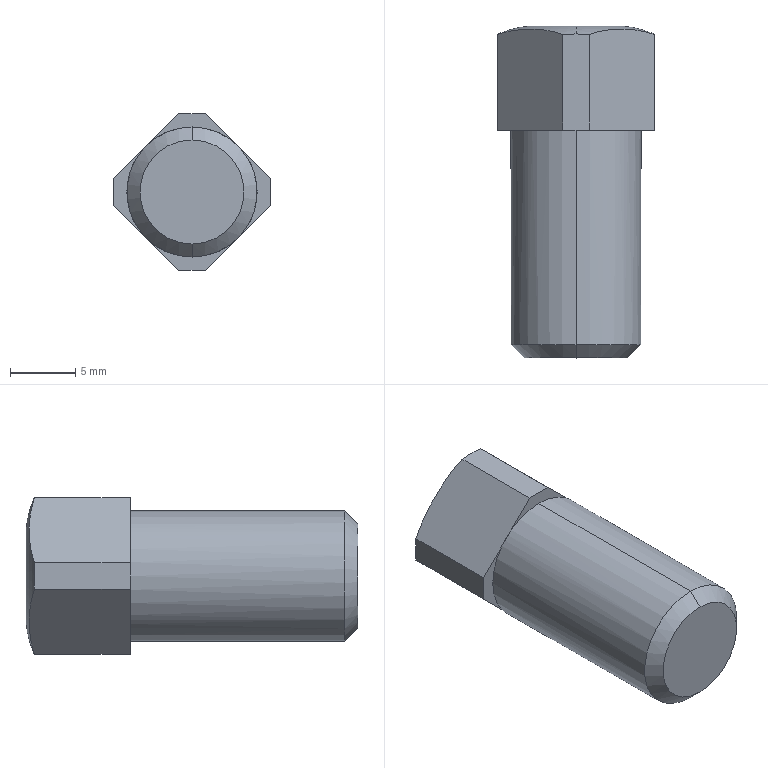Part | SolidWorks | features Chamfer 2, ICE 2, RevCut 1, Revolution 1 | 1 solid | 24 faces | box 12 x 25.5 x 12 mm | volume 2101 mm3 | plane 18 | cone 2 | torus 2 | cylinder 2 | commonest cylinder face diameters 10 x2
STEP:
#1=CARTESIAN_POINT('',(0.,-1.5,-4.));
#2=VERTEX_POINT('',#1);
#3=CARTESIAN_POINT('',(0.,-1.5,4.));
#4=VERTEX_POINT('',#3);
#5=CARTESIAN_POINT('',(0.,-1.5,0.));
#6=DIRECTION('',(0.,-1.,0.));
#7=DIRECTION('',(0.,0.,-1.));
#8=AXIS2_PLACEMENT_3D('',#5,#6,#7);
#9=CIRCLE('',#8,4.);
#10=EDGE_CURVE('',#2,#4,#9,.T.);
#11=ORIENTED_EDGE('',*,*,#10,.F.);
#12=CARTESIAN_POINT('',(0.,-0.5,-5.));
#13=VERTEX_POINT('',#12);
#14=CARTESIAN_POINT('',(0.,-1.5,-4.));
#15=DIRECTION('',(0.,0.7071,-0.7071));
#16=VECTOR('',#15,1000.);
#17=LINE('',#14,#16);
#18=EDGE_CURVE('',#2,#13,#17,.T.);
#19=ORIENTED_EDGE('',*,*,#18,.T.);
#20=CARTESIAN_POINT('',(0.,-0.5,5.));
#21=VERTEX_POINT('',#20);
#22=CARTESIAN_POINT('',(0.,-0.5,0.));
#23=DIRECTION('',(0.,1.,0.));
#24=DIRECTION('',(0.,0.,-1.));
#25=AXIS2_PLACEMENT_3D('',#22,#23,#24);
#26=CIRCLE('',#25,5.);
#27=EDGE_CURVE('',#21,#13,#26,.T.);
#28=ORIENTED_EDGE('',*,*,#27,.F.);
#29=CARTESIAN_POINT('',(0.,-1.5,4.));
#30=DIRECTION('',(0.,0.7071,0.7071));
#31=VECTOR('',#30,1000.);
#32=LINE('',#29,#31);
#33=EDGE_CURVE('',#4,#21,#32,.T.);
#34=ORIENTED_EDGE('',*,*,#33,.F.);
#35=EDGE_LOOP('',(#11,#19,#28,#34));
#36=FACE_OUTER_BOUND('',#35,.T.);
#37=CARTESIAN_POINT('',(0.,-1.5,0.));
#38=DIRECTION('',(0.,1.,0.));
#39=DIRECTION('',(0.,0.,1.));
#40=AXIS2_PLACEMENT_3D('',#37,#38,#39);
#41=CONICAL_SURFACE('',#40,4.,0.7854);
#42=ADVANCED_FACE('',(#36),#41,.T.);
#43=CARTESIAN_POINT('',(0.,24.,-3.5));
#44=VERTEX_POINT('',#43);
#45=CARTESIAN_POINT('',(0.,24.,3.5));
#46=VERTEX_POINT('',#45);
#47=CARTESIAN_POINT('',(0.,24.,0.));
#48=DIRECTION('',(0.,-1.,0.));
#49=DIRECTION('',(0.,0.,-1.));
#50=AXIS2_PLACEMENT_3D('',#47,#48,#49);
#51=CIRCLE('',#50,3.5);
#52=EDGE_CURVE('',#44,#46,#51,.T.);
#53=ORIENTED_EDGE('',*,*,#52,.T.);
#54=CARTESIAN_POINT('',(0.,23.385,6.));
#55=VERTEX_POINT('',#54);
#56=CARTESIAN_POINT('',(0.,16.602,3.006));
#57=DIRECTION('',(1.,0.,0.));
#58=DIRECTION('',(0.,0.,-1.));
#59=AXIS2_PLACEMENT_3D('',#56,#57,#58);
#60=CIRCLE('',#59,7.415);
#61=EDGE_CURVE('',#46,#55,#60,.T.);
#62=ORIENTED_EDGE('',*,*,#61,.T.);
#63=CARTESIAN_POINT('',(1.,23.348,6.));
#64=VERTEX_POINT('',#63);
#65=CARTESIAN_POINT('',(0.,23.385,6.));
#66=CARTESIAN_POINT('',(0.1677,23.385,6.));
#67=CARTESIAN_POINT('',(0.5021,23.379,6.));
#68=CARTESIAN_POINT('',(0.8344,23.36,6.));
#69=CARTESIAN_POINT('',(1.,23.348,6.));
#70=B_SPLINE_CURVE_WITH_KNOTS('',3,(#65,#66,#67,#68,#69),.UNSPECIFIED.,.F.,.F.,(4,1,4),(0.,0.0004963,0.0009926),.UNSPECIFIED.);
#71=EDGE_CURVE('',#55,#64,#70,.T.);
#72=ORIENTED_EDGE('',*,*,#71,.T.);
#73=CARTESIAN_POINT('',(6.,23.348,1.));
#74=VERTEX_POINT('',#73);
#75=CARTESIAN_POINT('',(1.,23.348,6.));
#76=CARTESIAN_POINT('',(1.411,23.502,5.589));
#77=CARTESIAN_POINT('',(1.825,23.602,5.175));
#78=CARTESIAN_POINT('',(2.657,23.729,4.343));
#79=CARTESIAN_POINT('',(3.075,23.757,3.925));
#80=CARTESIAN_POINT('',(3.915,23.757,3.085));
#81=CARTESIAN_POINT('',(4.339,23.73,2.661));
#82=CARTESIAN_POINT('',(5.176,23.602,1.824));
#83=CARTESIAN_POINT('',(5.591,23.501,1.409));
#84=CARTESIAN_POINT('',(6.,23.348,1.));
#85=B_SPLINE_CURVE_WITH_KNOTS('',3,(#75,#76,#77,#78,#79,#80,#81,#82,#83,#84),.UNSPECIFIED.,.F.,.F.,(4,2,2,2,4),(0.000000288,0.001776,0.003551,0.005327,0.007102),.UNSPECIFIED.);
#86=EDGE_CURVE('',#64,#74,#85,.T.);
#87=ORIENTED_EDGE('',*,*,#86,.T.);
#88=CARTESIAN_POINT('',(6.,23.348,-1.));
#89=VERTEX_POINT('',#88);
#90=CARTESIAN_POINT('',(6.,23.348,1.));
#91=CARTESIAN_POINT('',(6.,23.373,0.6665));
#92=CARTESIAN_POINT('',(6.,23.385,0.3303));
#93=CARTESIAN_POINT('',(6.,23.385,-0.3379));
#94=CARTESIAN_POINT('',(6.,23.373,-0.67));
#95=CARTESIAN_POINT('',(6.,23.348,-1.));
#96=B_SPLINE_CURVE_WITH_KNOTS('',3,(#90,#91,#92,#93,#94,#95),.UNSPECIFIED.,.F.,.F.,(4,2,4),(0.04716,0.04814,0.04913),.UNSPECIFIED.);
#97=EDGE_CURVE('',#74,#89,#96,.T.);
#98=ORIENTED_EDGE('',*,*,#97,.T.);
#99=CARTESIAN_POINT('',(1.,23.348,-6.));
#100=VERTEX_POINT('',#99);
#101=CARTESIAN_POINT('',(6.,23.348,-1.));
#102=CARTESIAN_POINT('',(5.589,23.502,-1.411));
#103=CARTESIAN_POINT('',(5.175,23.602,-1.825));
#104=CARTESIAN_POINT('',(4.343,23.729,-2.657));
#105=CARTESIAN_POINT('',(3.925,23.757,-3.075));
#106=CARTESIAN_POINT('',(3.085,23.757,-3.915));
#107=CARTESIAN_POINT('',(2.661,23.73,-4.339));
#108=CARTESIAN_POINT('',(1.824,23.602,-5.176));
#109=CARTESIAN_POINT('',(1.409,23.501,-5.591));
#110=CARTESIAN_POINT('',(1.,23.348,-6.));
#111=B_SPLINE_CURVE_WITH_KNOTS('',3,(#101,#102,#103,#104,#105,#106,#107,#108,#109,#110),.UNSPECIFIED.,.F.,.F.,(4,2,2,2,4),(0.000000288,0.001776,0.003551,0.005327,0.007102),.UNSPECIFIED.);
#112=EDGE_CURVE('',#89,#100,#111,.T.);
#113=ORIENTED_EDGE('',*,*,#112,.T.);
#114=CARTESIAN_POINT('',(0.,23.385,-6.));
#115=VERTEX_POINT('',#114);
#116=CARTESIAN_POINT('',(1.,23.348,-6.));
#117=CARTESIAN_POINT('',(0.8339,23.36,-6.));
#118=CARTESIAN_POINT('',(0.6675,23.37,-6.));
#119=CARTESIAN_POINT('',(0.3342,23.382,-6.));
#120=CARTESIAN_POINT('',(0.1664,23.385,-6.));
#121=CARTESIAN_POINT('',(0.,23.385,-6.));
#122=B_SPLINE_CURVE_WITH_KNOTS('',3,(#116,#117,#118,#119,#120,#121),.UNSPECIFIED.,.F.,.F.,(4,2,4),(0.04716,0.04765,0.04814),.UNSPECIFIED.);
#123=EDGE_CURVE('',#100,#115,#122,.T.);
#124=ORIENTED_EDGE('',*,*,#123,.T.);
#125=CARTESIAN_POINT('',(0.,16.602,-3.006));
#126=DIRECTION('',(-1.,0.,0.));
#127=DIRECTION('',(0.,0.,1.));
#128=AXIS2_PLACEMENT_3D('',#125,#126,#127);
#129=CIRCLE('',#128,7.415);
#130=EDGE_CURVE('',#44,#115,#129,.T.);
#131=ORIENTED_EDGE('',*,*,#130,.F.);
#132=EDGE_LOOP('',(#53,#62,#72,#87,#98,#113,#124,#131));
#133=FACE_OUTER_BOUND('',#132,.T.);
#134=CARTESIAN_POINT('',(0.,16.602,0.));
#135=DIRECTION('',(0.,-1.,0.));
#136=DIRECTION('',(0.,0.,-1.));
#137=AXIS2_PLACEMENT_3D('',#134,#135,#136);
#138=TOROIDAL_SURFACE('',#137,3.006,7.415);
#139=ADVANCED_FACE('',(#133),#138,.T.);
#140=CARTESIAN_POINT('',(3.,16.,4.));
#141=VERTEX_POINT('',#140);
#142=CARTESIAN_POINT('',(0.,16.,5.));
#143=VERTEX_POINT('',#142);
#144=CARTESIAN_POINT('',(0.,16.,0.));
#145=DIRECTION('',(0.,-1.,0.));
#146=DIRECTION('',(0.,0.,-1.));
#147=AXIS2_PLACEMENT_3D('',#144,#145,#146);
#148=CIRCLE('',#147,5.);
#149=EDGE_CURVE('',#141,#143,#148,.T.);
#150=ORIENTED_EDGE('',*,*,#149,.T.);
#151=CARTESIAN_POINT('',(0.,0.,5.));
#152=DIRECTION('',(0.,-1.,0.));
#153=VECTOR('',#152,1000.);
#154=LINE('',#151,#153);
#155=EDGE_CURVE('',#143,#21,#154,.T.);
#156=ORIENTED_EDGE('',*,*,#155,.T.);
#157=ORIENTED_EDGE('',*,*,#27,.T.);
#158=CARTESIAN_POINT('',(0.,16.,-5.));
#159=VERTEX_POINT('',#158);
#160=CARTESIAN_POINT('',(0.,0.,-5.));
#161=DIRECTION('',(0.,-1.,0.));
#162=VECTOR('',#161,1000.);
#163=LINE('',#160,#162);
#164=EDGE_CURVE('',#159,#13,#163,.T.);
#165=ORIENTED_EDGE('',*,*,#164,.F.);
#166=CARTESIAN_POINT('',(3.,16.,-4.));
#167=VERTEX_POINT('',#166);
#168=CARTESIAN_POINT('',(0.,16.,0.));
#169=DIRECTION('',(0.,-1.,0.));
#170=DIRECTION('',(0.,0.,-1.));
#171=AXIS2_PLACEMENT_3D('',#168,#169,#170);
#172=CIRCLE('',#171,5.);
#173=EDGE_CURVE('',#159,#167,#172,.T.);
#174=ORIENTED_EDGE('',*,*,#173,.T.);
#175=CARTESIAN_POINT('',(4.,16.,-3.));
#176=VERTEX_POINT('',#175);
#177=CARTESIAN_POINT('',(0.,16.,0.));
#178=DIRECTION('',(0.,-1.,0.));
#179=DIRECTION('',(0.,0.,-1.));
#180=AXIS2_PLACEMENT_3D('',#177,#178,#179);
#181=CIRCLE('',#180,5.);
#182=EDGE_CURVE('',#167,#176,#181,.T.);
#183=ORIENTED_EDGE('',*,*,#182,.T.);
#184=CARTESIAN_POINT('',(4.,16.,3.));
#185=VERTEX_POINT('',#184);
#186=CARTESIAN_POINT('',(0.,16.,0.));
#187=DIRECTION('',(0.,-1.,0.));
#188=DIRECTION('',(0.,0.,-1.));
#189=AXIS2_PLACEMENT_3D('',#186,#187,#188);
#190=CIRCLE('',#189,5.);
#191=EDGE_CURVE('',#176,#185,#190,.T.);
#192=ORIENTED_EDGE('',*,*,#191,.T.);
#193=CARTESIAN_POINT('',(0.,16.,0.));
#194=DIRECTION('',(0.,-1.,0.));
#195=DIRECTION('',(0.,0.,-1.));
#196=AXIS2_PLACEMENT_3D('',#193,#194,#195);
#197=CIRCLE('',#196,5.);
#198=EDGE_CURVE('',#185,#141,#197,.T.);
#199=ORIENTED_EDGE('',*,*,#198,.T.);
#200=EDGE_LOOP('',(#150,#156,#157,#165,#174,#183,#192,#199));
#201=FACE_OUTER_BOUND('',#200,.T.);
#202=CARTESIAN_POINT('',(0.,0.,0.));
#203=DIRECTION('',(0.,-1.,0.));
#204=DIRECTION('',(0.,0.,-1.));
#205=AXIS2_PLACEMENT_3D('',#202,#203,#204);
#206=CYLINDRICAL_SURFACE('',#205,5.);
#207=ADVANCED_FACE('',(#201),#206,.T.);
#208=CARTESIAN_POINT('',(-3.,16.,-4.));
#209=VERTEX_POINT('',#208);
#210=CARTESIAN_POINT('',(0.,16.,0.));
#211=DIRECTION('',(0.,-1.,0.));
#212=DIRECTION('',(0.,0.,-1.));
#213=AXIS2_PLACEMENT_3D('',#210,#211,#212);
#214=CIRCLE('',#213,5.);
#215=EDGE_CURVE('',#209,#159,#214,.T.);
#216=ORIENTED_EDGE('',*,*,#215,.F.);
#217=CARTESIAN_POINT('',(-1.,16.,-6.));
#218=VERTEX_POINT('',#217);
#219=CARTESIAN_POINT('',(-1.,16.,-6.));
#220=DIRECTION('',(-0.7071,0.,0.7071));
#221=VECTOR('',#220,1000.);
#222=LINE('',#219,#221);
#223=EDGE_CURVE('',#218,#209,#222,.T.);
#224=ORIENTED_EDGE('',*,*,#223,.F.);
#225=CARTESIAN_POINT('',(1.,16.,-6.));
#226=VERTEX_POINT('',#225);
#227=CARTESIAN_POINT('',(-1.,16.,-6.));
#228=DIRECTION('',(-1.,0.,0.));
#229=VECTOR('',#228,1000.);
#230=LINE('',#227,#229);
#231=EDGE_CURVE('',#226,#218,#230,.T.);
#232=ORIENTED_EDGE('',*,*,#231,.F.);
#233=CARTESIAN_POINT('',(6.,16.,-1.));
#234=DIRECTION('',(-0.7071,0.,-0.7071));
#235=VECTOR('',#234,1000.);
#236=LINE('',#233,#235);
#237=EDGE_CURVE('',#167,#226,#236,.T.);
#238=ORIENTED_EDGE('',*,*,#237,.F.);
#239=ORIENTED_EDGE('',*,*,#173,.F.);
#240=EDGE_LOOP('',(#216,#224,#232,#238,#239));
#241=FACE_OUTER_BOUND('',#240,.T.);
#242=CARTESIAN_POINT('',(10.,16.,0.));
#243=DIRECTION('',(0.,-1.,0.));
#244=DIRECTION('',(0.,0.,-1.));
#245=AXIS2_PLACEMENT_3D('',#242,#243,#244);
#246=PLANE('',#245);
#247=ADVANCED_FACE('',(#241),#246,.T.);
#248=ORIENTED_EDGE('',*,*,#191,.F.);
#249=CARTESIAN_POINT('',(6.,16.,-1.));
#250=VERTEX_POINT('',#249);
#251=CARTESIAN_POINT('',(6.,16.,-1.));
#252=DIRECTION('',(-0.7071,0.,-0.7071));
#253=VECTOR('',#252,1000.);
#254=LINE('',#251,#253);
#255=EDGE_CURVE('',#250,#176,#254,.T.);
#256=ORIENTED_EDGE('',*,*,#255,.F.);
#257=CARTESIAN_POINT('',(6.,16.,1.));
#258=VERTEX_POINT('',#257);
#259=CARTESIAN_POINT('',(6.,16.,-1.));
#260=DIRECTION('',(0.,0.,-1.));
#261=VECTOR('',#260,1000.);
#262=LINE('',#259,#261);
#263=EDGE_CURVE('',#258,#250,#262,.T.);
#264=ORIENTED_EDGE('',*,*,#263,.F.);
#265=CARTESIAN_POINT('',(6.,16.,1.));
#266=DIRECTION('',(0.7071,0.,-0.7071));
#267=VECTOR('',#266,1000.);
#268=LINE('',#265,#267);
#269=EDGE_CURVE('',#185,#258,#268,.T.);
#270=ORIENTED_EDGE('',*,*,#269,.F.);
#271=EDGE_LOOP('',(#248,#256,#264,#270));
#272=FACE_OUTER_BOUND('',#271,.T.);
#273=CARTESIAN_POINT('',(10.,16.,0.));
#274=DIRECTION('',(0.,-1.,0.));
#275=DIRECTION('',(0.,0.,-1.));
#276=AXIS2_PLACEMENT_3D('',#273,#274,#275);
#277=PLANE('',#276);
#278=ADVANCED_FACE('',(#272),#277,.T.);
#279=ORIENTED_EDGE('',*,*,#149,.F.);
#280=CARTESIAN_POINT('',(1.,16.,6.));
#281=VERTEX_POINT('',#280);
#282=CARTESIAN_POINT('',(6.,16.,1.));
#283=DIRECTION('',(0.7071,0.,-0.7071));
#284=VECTOR('',#283,1000.);
#285=LINE('',#282,#284);
#286=EDGE_CURVE('',#281,#141,#285,.T.);
#287=ORIENTED_EDGE('',*,*,#286,.F.);
#288=CARTESIAN_POINT('',(-1.,16.,6.));
#289=VERTEX_POINT('',#288);
#290=CARTESIAN_POINT('',(-1.,16.,6.));
#291=DIRECTION('',(1.,0.,0.));
#292=VECTOR('',#291,1000.);
#293=LINE('',#290,#292);
#294=EDGE_CURVE('',#289,#281,#293,.T.);
#295=ORIENTED_EDGE('',*,*,#294,.F.);
#296=CARTESIAN_POINT('',(-3.,16.,4.));
#297=VERTEX_POINT('',#296);
#298=CARTESIAN_POINT('',(-1.,16.,6.));
#299=DIRECTION('',(0.7071,0.,0.7071));
#300=VECTOR('',#299,1000.);
#301=LINE('',#298,#300);
#302=EDGE_CURVE('',#297,#289,#301,.T.);
#303=ORIENTED_EDGE('',*,*,#302,.F.);
#304=CARTESIAN_POINT('',(0.,16.,0.));
#305=DIRECTION('',(0.,-1.,0.));
#306=DIRECTION('',(0.,0.,-1.));
#307=AXIS2_PLACEMENT_3D('',#304,#305,#306);
#308=CIRCLE('',#307,5.);
#309=EDGE_CURVE('',#143,#297,#308,.T.);
#310=ORIENTED_EDGE('',*,*,#309,.F.);
#311=EDGE_LOOP('',(#279,#287,#295,#303,#310));
#312=FACE_OUTER_BOUND('',#311,.T.);
#313=CARTESIAN_POINT('',(10.,16.,0.));
#314=DIRECTION('',(0.,-1.,0.));
#315=DIRECTION('',(0.,0.,-1.));
#316=AXIS2_PLACEMENT_3D('',#313,#314,#315);
#317=PLANE('',#316);
#318=ADVANCED_FACE('',(#312),#317,.T.);
#319=CARTESIAN_POINT('',(-6.,16.,-1.));
#320=VERTEX_POINT('',#319);
#321=CARTESIAN_POINT('',(-6.,16.,1.));
#322=VERTEX_POINT('',#321);
#323=CARTESIAN_POINT('',(-6.,16.,-1.));
#324=DIRECTION('',(0.,0.,1.));
#325=VECTOR('',#324,1000.);
#326=LINE('',#323,#325);
#327=EDGE_CURVE('',#320,#322,#326,.T.);
#328=ORIENTED_EDGE('',*,*,#327,.F.);
#329=CARTESIAN_POINT('',(-4.,16.,-3.));
#330=VERTEX_POINT('',#329);
#331=CARTESIAN_POINT('',(-1.,16.,-6.));
#332=DIRECTION('',(-0.7071,0.,0.7071));
#333=VECTOR('',#332,1000.);
#334=LINE('',#331,#333);
#335=EDGE_CURVE('',#330,#320,#334,.T.);
#336=ORIENTED_EDGE('',*,*,#335,.F.);
#337=CARTESIAN_POINT('',(-4.,16.,3.));
#338=VERTEX_POINT('',#337);
#339=CARTESIAN_POINT('',(0.,16.,0.));
#340=DIRECTION('',(0.,-1.,0.));
#341=DIRECTION('',(0.,0.,-1.));
#342=AXIS2_PLACEMENT_3D('',#339,#340,#341);
#343=CIRCLE('',#342,5.);
#344=EDGE_CURVE('',#338,#330,#343,.T.);
#345=ORIENTED_EDGE('',*,*,#344,.F.);
#346=CARTESIAN_POINT('',(-1.,16.,6.));
#347=DIRECTION('',(0.7071,0.,0.7071));
#348=VECTOR('',#347,1000.);
#349=LINE('',#346,#348);
#350=EDGE_CURVE('',#322,#338,#349,.T.);
#351=ORIENTED_EDGE('',*,*,#350,.F.);
#352=EDGE_LOOP('',(#328,#336,#345,#351));
#353=FACE_OUTER_BOUND('',#352,.T.);
#354=CARTESIAN_POINT('',(10.,16.,0.));
#355=DIRECTION('',(0.,-1.,0.));
#356=DIRECTION('',(0.,0.,-1.));
#357=AXIS2_PLACEMENT_3D('',#354,#355,#356);
#358=PLANE('',#357);
#359=ADVANCED_FACE('',(#353),#358,.T.);
#360=ORIENTED_EDGE('',*,*,#155,.F.);
#361=ORIENTED_EDGE('',*,*,#309,.T.);
#362=CARTESIAN_POINT('',(0.,16.,0.));
#363=DIRECTION('',(0.,-1.,0.));
#364=DIRECTION('',(0.,0.,-1.));
#365=AXIS2_PLACEMENT_3D('',#362,#363,#364);
#366=CIRCLE('',#365,5.);
#367=EDGE_CURVE('',#297,#338,#366,.T.);
#368=ORIENTED_EDGE('',*,*,#367,.T.);
#369=ORIENTED_EDGE('',*,*,#344,.T.);
#370=CARTESIAN_POINT('',(0.,16.,0.));
#371=DIRECTION('',(0.,-1.,0.));
#372=DIRECTION('',(0.,0.,-1.));
#373=AXIS2_PLACEMENT_3D('',#370,#371,#372);
#374=CIRCLE('',#373,5.);
#375=EDGE_CURVE('',#330,#209,#374,.T.);
#376=ORIENTED_EDGE('',*,*,#375,.T.);
#377=ORIENTED_EDGE('',*,*,#215,.T.);
#378=ORIENTED_EDGE('',*,*,#164,.T.);
#379=CARTESIAN_POINT('',(0.,-0.5,0.));
#380=DIRECTION('',(0.,1.,0.));
#381=DIRECTION('',(0.,0.,-1.));
#382=AXIS2_PLACEMENT_3D('',#379,#380,#381);
#383=CIRCLE('',#382,5.);
#384=EDGE_CURVE('',#13,#21,#383,.T.);
#385=ORIENTED_EDGE('',*,*,#384,.T.);
#386=EDGE_LOOP('',(#360,#361,#368,#369,#376,#377,#378,#385));
#387=FACE_OUTER_BOUND('',#386,.T.);
#388=CARTESIAN_POINT('',(0.,0.,0.));
#389=DIRECTION('',(0.,-1.,0.));
#390=DIRECTION('',(0.,0.,-1.));
#391=AXIS2_PLACEMENT_3D('',#388,#389,#390);
#392=CYLINDRICAL_SURFACE('',#391,5.);
#393=ADVANCED_FACE('',(#387),#392,.T.);
#394=ORIENTED_EDGE('',*,*,#375,.F.);
#395=CARTESIAN_POINT('',(-1.,16.,-6.));
#396=DIRECTION('',(-0.7071,0.,0.7071));
#397=VECTOR('',#396,1000.);
#398=LINE('',#395,#397);
#399=EDGE_CURVE('',#209,#330,#398,.T.);
#400=ORIENTED_EDGE('',*,*,#399,.F.);
#401=EDGE_LOOP('',(#394,#400));
#402=FACE_OUTER_BOUND('',#401,.T.);
#403=CARTESIAN_POINT('',(10.,16.,0.));
#404=DIRECTION('',(0.,-1.,0.));
#405=DIRECTION('',(0.,0.,-1.));
#406=AXIS2_PLACEMENT_3D('',#403,#404,#405);
#407=PLANE('',#406);
#408=ADVANCED_FACE('',(#402),#407,.F.);
#409=ORIENTED_EDGE('',*,*,#367,.F.);
#410=CARTESIAN_POINT('',(-1.,16.,6.));
#411=DIRECTION('',(0.7071,0.,0.7071));
#412=VECTOR('',#411,1000.);
#413=LINE('',#410,#412);
#414=EDGE_CURVE('',#338,#297,#413,.T.);
#415=ORIENTED_EDGE('',*,*,#414,.F.);
#416=EDGE_LOOP('',(#409,#415));
#417=FACE_OUTER_BOUND('',#416,.T.);
#418=CARTESIAN_POINT('',(10.,16.,0.));
#419=DIRECTION('',(0.,-1.,0.));
#420=DIRECTION('',(0.,0.,-1.));
#421=AXIS2_PLACEMENT_3D('',#418,#419,#420);
#422=PLANE('',#421);
#423=ADVANCED_FACE('',(#417),#422,.F.);
#424=ORIENTED_EDGE('',*,*,#198,.F.);
#425=CARTESIAN_POINT('',(6.,16.,1.));
#426=DIRECTION('',(0.7071,0.,-0.7071));
#427=VECTOR('',#426,1000.);
#428=LINE('',#425,#427);
#429=EDGE_CURVE('',#141,#185,#428,.T.);
#430=ORIENTED_EDGE('',*,*,#429,.F.);
#431=EDGE_LOOP('',(#424,#430));
#432=FACE_OUTER_BOUND('',#431,.T.);
#433=CARTESIAN_POINT('',(10.,16.,0.));
#434=DIRECTION('',(0.,-1.,0.));
#435=DIRECTION('',(0.,0.,-1.));
#436=AXIS2_PLACEMENT_3D('',#433,#434,#435);
#437=PLANE('',#436);
#438=ADVANCED_FACE('',(#432),#437,.F.);
#439=CARTESIAN_POINT('',(-1.,23.348,-6.));
#440=VERTEX_POINT('',#439);
#441=CARTESIAN_POINT('',(-6.,23.348,-1.));
#442=VERTEX_POINT('',#441);
#443=CARTESIAN_POINT('',(-1.,23.348,-6.));
#444=CARTESIAN_POINT('',(-1.411,23.502,-5.589));
#445=CARTESIAN_POINT('',(-1.825,23.602,-5.175));
#446=CARTESIAN_POINT('',(-2.657,23.729,-4.343));
#447=CARTESIAN_POINT('',(-3.075,23.757,-3.925));
#448=CARTESIAN_POINT('',(-3.915,23.757,-3.085));
#449=CARTESIAN_POINT('',(-4.339,23.73,-2.661));
#450=CARTESIAN_POINT('',(-5.176,23.602,-1.824));
#451=CARTESIAN_POINT('',(-5.591,23.501,-1.409));
#452=CARTESIAN_POINT('',(-6.,23.348,-1.));
#453=B_SPLINE_CURVE_WITH_KNOTS('',3,(#443,#444,#445,#446,#447,#448,#449,#450,#451,#452),.UNSPECIFIED.,.F.,.F.,(4,2,2,2,4),(0.000000288,0.001776,0.003551,0.005327,0.007102),.UNSPECIFIED.);
#454=EDGE_CURVE('',#440,#442,#453,.T.);
#455=ORIENTED_EDGE('',*,*,#454,.F.);
#456=CARTESIAN_POINT('',(-1.,-17.879,-6.));
#457=DIRECTION('',(0.,1.,0.));
#458=VECTOR('',#457,1000.);
#459=LINE('',#456,#458);
#460=EDGE_CURVE('',#218,#440,#459,.T.);
#461=ORIENTED_EDGE('',*,*,#460,.F.);
#462=ORIENTED_EDGE('',*,*,#223,.T.);
#463=ORIENTED_EDGE('',*,*,#399,.T.);
#464=ORIENTED_EDGE('',*,*,#335,.T.);
#465=CARTESIAN_POINT('',(-6.,-17.879,-1.));
#466=DIRECTION('',(0.,1.,0.));
#467=VECTOR('',#466,1000.);
#468=LINE('',#465,#467);
#469=EDGE_CURVE('',#320,#442,#468,.T.);
#470=ORIENTED_EDGE('',*,*,#469,.T.);
#471=EDGE_LOOP('',(#455,#461,#462,#463,#464,#470));
#472=FACE_OUTER_BOUND('',#471,.T.);
#473=CARTESIAN_POINT('',(-1.,-17.879,-6.));
#474=DIRECTION('',(-0.7071,0.,-0.7071));
#475=DIRECTION('',(-0.7071,0.,0.7071));
#476=AXIS2_PLACEMENT_3D('',#473,#474,#475);
#477=PLANE('',#476);
#478=ADVANCED_FACE('',(#472),#477,.T.);
#479=ORIENTED_EDGE('',*,*,#123,.F.);
#480=CARTESIAN_POINT('',(1.,-17.879,-6.));
#481=DIRECTION('',(0.,1.,0.));
#482=VECTOR('',#481,1000.);
#483=LINE('',#480,#482);
#484=EDGE_CURVE('',#226,#100,#483,.T.);
#485=ORIENTED_EDGE('',*,*,#484,.F.);
#486=ORIENTED_EDGE('',*,*,#231,.T.);
#487=ORIENTED_EDGE('',*,*,#460,.T.);
#488=CARTESIAN_POINT('',(0.,23.385,-6.));
#489=CARTESIAN_POINT('',(-0.1677,23.385,-6.));
#490=CARTESIAN_POINT('',(-0.5021,23.379,-6.));
#491=CARTESIAN_POINT('',(-0.8344,23.36,-6.));
#492=CARTESIAN_POINT('',(-1.,23.348,-6.));
#493=B_SPLINE_CURVE_WITH_KNOTS('',3,(#488,#489,#490,#491,#492),.UNSPECIFIED.,.F.,.F.,(4,1,4),(0.,0.0004963,0.0009926),.UNSPECIFIED.);
#494=EDGE_CURVE('',#115,#440,#493,.T.);
#495=ORIENTED_EDGE('',*,*,#494,.F.);
#496=EDGE_LOOP('',(#479,#485,#486,#487,#495));
#497=FACE_OUTER_BOUND('',#496,.T.);
#498=CARTESIAN_POINT('',(-1.,-17.879,-6.));
#499=DIRECTION('',(0.,0.,-1.));
#500=DIRECTION('',(-1.,0.,0.));
#501=AXIS2_PLACEMENT_3D('',#498,#499,#500);
#502=PLANE('',#501);
#503=ADVANCED_FACE('',(#497),#502,.T.);
#504=ORIENTED_EDGE('',*,*,#112,.F.);
#505=CARTESIAN_POINT('',(6.,-17.879,-1.));
#506=DIRECTION('',(0.,1.,0.));
#507=VECTOR('',#506,1000.);
#508=LINE('',#505,#507);
#509=EDGE_CURVE('',#250,#89,#508,.T.);
#510=ORIENTED_EDGE('',*,*,#509,.F.);
#511=ORIENTED_EDGE('',*,*,#255,.T.);
#512=CARTESIAN_POINT('',(6.,16.,-1.));
#513=DIRECTION('',(-0.7071,0.,-0.7071));
#514=VECTOR('',#513,1000.);
#515=LINE('',#512,#514);
#516=EDGE_CURVE('',#176,#167,#515,.T.);
#517=ORIENTED_EDGE('',*,*,#516,.T.);
#518=ORIENTED_EDGE('',*,*,#237,.T.);
#519=ORIENTED_EDGE('',*,*,#484,.T.);
#520=EDGE_LOOP('',(#504,#510,#511,#517,#518,#519));
#521=FACE_OUTER_BOUND('',#520,.T.);
#522=CARTESIAN_POINT('',(6.,-17.879,-1.));
#523=DIRECTION('',(0.7071,0.,-0.7071));
#524=DIRECTION('',(-0.7071,0.,-0.7071));
#525=AXIS2_PLACEMENT_3D('',#522,#523,#524);
#526=PLANE('',#525);
#527=ADVANCED_FACE('',(#521),#526,.T.);
#528=ORIENTED_EDGE('',*,*,#97,.F.);
#529=CARTESIAN_POINT('',(6.,-17.879,1.));
#530=DIRECTION('',(0.,1.,0.));
#531=VECTOR('',#530,1000.);
#532=LINE('',#529,#531);
#533=EDGE_CURVE('',#258,#74,#532,.T.);
#534=ORIENTED_EDGE('',*,*,#533,.F.);
#535=ORIENTED_EDGE('',*,*,#263,.T.);
#536=ORIENTED_EDGE('',*,*,#509,.T.);
#537=EDGE_LOOP('',(#528,#534,#535,#536));
#538=FACE_OUTER_BOUND('',#537,.T.);
#539=CARTESIAN_POINT('',(6.,-17.879,-1.));
#540=DIRECTION('',(1.,0.,0.));
#541=DIRECTION('',(0.,0.,-1.));
#542=AXIS2_PLACEMENT_3D('',#539,#540,#541);
#543=PLANE('',#542);
#544=ADVANCED_FACE('',(#538),#543,.T.);
#545=ORIENTED_EDGE('',*,*,#86,.F.);
#546=CARTESIAN_POINT('',(1.,-17.879,6.));
#547=DIRECTION('',(0.,1.,0.));
#548=VECTOR('',#547,1000.);
#549=LINE('',#546,#548);
#550=EDGE_CURVE('',#281,#64,#549,.T.);
#551=ORIENTED_EDGE('',*,*,#550,.F.);
#552=ORIENTED_EDGE('',*,*,#286,.T.);
#553=ORIENTED_EDGE('',*,*,#429,.T.);
#554=ORIENTED_EDGE('',*,*,#269,.T.);
#555=ORIENTED_EDGE('',*,*,#533,.T.);
#556=EDGE_LOOP('',(#545,#551,#552,#553,#554,#555));
#557=FACE_OUTER_BOUND('',#556,.T.);
#558=CARTESIAN_POINT('',(6.,-17.879,1.));
#559=DIRECTION('',(0.7071,0.,0.7071));
#560=DIRECTION('',(0.7071,0.,-0.7071));
#561=AXIS2_PLACEMENT_3D('',#558,#559,#560);
#562=PLANE('',#561);
#563=ADVANCED_FACE('',(#557),#562,.T.);
#564=CARTESIAN_POINT('',(-1.,23.348,6.));
#565=VERTEX_POINT('',#564);
#566=CARTESIAN_POINT('',(-1.,23.348,6.));
#567=CARTESIAN_POINT('',(-0.8339,23.36,6.));
#568=CARTESIAN_POINT('',(-0.6675,23.37,6.));
#569=CARTESIAN_POINT('',(-0.3342,23.382,6.));
#570=CARTESIAN_POINT('',(-0.1664,23.385,6.));
#571=CARTESIAN_POINT('',(0.,23.385,6.));
#572=B_SPLINE_CURVE_WITH_KNOTS('',3,(#566,#567,#568,#569,#570,#571),.UNSPECIFIED.,.F.,.F.,(4,2,4),(0.04716,0.04765,0.04814),.UNSPECIFIED.);
#573=EDGE_CURVE('',#565,#55,#572,.T.);
#574=ORIENTED_EDGE('',*,*,#573,.F.);
#575=CARTESIAN_POINT('',(-1.,-17.879,6.));
#576=DIRECTION('',(0.,1.,0.));
#577=VECTOR('',#576,1000.);
#578=LINE('',#575,#577);
#579=EDGE_CURVE('',#289,#565,#578,.T.);
#580=ORIENTED_EDGE('',*,*,#579,.F.);
#581=ORIENTED_EDGE('',*,*,#294,.T.);
#582=ORIENTED_EDGE('',*,*,#550,.T.);
#583=ORIENTED_EDGE('',*,*,#71,.F.);
#584=EDGE_LOOP('',(#574,#580,#581,#582,#583));
#585=FACE_OUTER_BOUND('',#584,.T.);
#586=CARTESIAN_POINT('',(-1.,-17.879,6.));
#587=DIRECTION('',(0.,0.,1.));
#588=DIRECTION('',(1.,0.,0.));
#589=AXIS2_PLACEMENT_3D('',#586,#587,#588);
#590=PLANE('',#589);
#591=ADVANCED_FACE('',(#585),#590,.T.);
#592=CARTESIAN_POINT('',(-6.,23.348,1.));
#593=VERTEX_POINT('',#592);
#594=CARTESIAN_POINT('',(-6.,23.348,1.));
#595=CARTESIAN_POINT('',(-5.589,23.502,1.411));
#596=CARTESIAN_POINT('',(-5.175,23.602,1.825));
#597=CARTESIAN_POINT('',(-4.343,23.729,2.657));
#598=CARTESIAN_POINT('',(-3.925,23.757,3.075));
#599=CARTESIAN_POINT('',(-3.085,23.757,3.915));
#600=CARTESIAN_POINT('',(-2.661,23.73,4.339));
#601=CARTESIAN_POINT('',(-1.824,23.602,5.176));
#602=CARTESIAN_POINT('',(-1.409,23.501,5.591));
#603=CARTESIAN_POINT('',(-1.,23.348,6.));
#604=B_SPLINE_CURVE_WITH_KNOTS('',3,(#594,#595,#596,#597,#598,#599,#600,#601,#602,#603),.UNSPECIFIED.,.F.,.F.,(4,2,2,2,4),(0.000000288,0.001776,0.003551,0.005327,0.007102),.UNSPECIFIED.);
#605=EDGE_CURVE('',#593,#565,#604,.T.);
#606=ORIENTED_EDGE('',*,*,#605,.F.);
#607=CARTESIAN_POINT('',(-6.,-17.879,1.));
#608=DIRECTION('',(0.,1.,0.));
#609=VECTOR('',#608,1000.);
#610=LINE('',#607,#609);
#611=EDGE_CURVE('',#322,#593,#610,.T.);
#612=ORIENTED_EDGE('',*,*,#611,.F.);
#613=ORIENTED_EDGE('',*,*,#350,.T.);
#614=ORIENTED_EDGE('',*,*,#414,.T.);
#615=ORIENTED_EDGE('',*,*,#302,.T.);
#616=ORIENTED_EDGE('',*,*,#579,.T.);
#617=EDGE_LOOP('',(#606,#612,#613,#614,#615,#616));
#618=FACE_OUTER_BOUND('',#617,.T.);
#619=CARTESIAN_POINT('',(-1.,-17.879,6.));
#620=DIRECTION('',(-0.7071,0.,0.7071));
#621=DIRECTION('',(0.7071,0.,0.7071));
#622=AXIS2_PLACEMENT_3D('',#619,#620,#621);
#623=PLANE('',#622);
#624=ADVANCED_FACE('',(#618),#623,.T.);
#625=CARTESIAN_POINT('',(-6.,23.348,-1.));
#626=CARTESIAN_POINT('',(-6.,23.373,-0.6665));
#627=CARTESIAN_POINT('',(-6.,23.385,-0.3303));
#628=CARTESIAN_POINT('',(-6.,23.385,0.3379));
#629=CARTESIAN_POINT('',(-6.,23.373,0.67));
#630=CARTESIAN_POINT('',(-6.,23.348,1.));
#631=B_SPLINE_CURVE_WITH_KNOTS('',3,(#625,#626,#627,#628,#629,#630),.UNSPECIFIED.,.F.,.F.,(4,2,4),(0.04716,0.04814,0.04913),.UNSPECIFIED.);
#632=EDGE_CURVE('',#442,#593,#631,.T.);
#633=ORIENTED_EDGE('',*,*,#632,.F.);
#634=ORIENTED_EDGE('',*,*,#469,.F.);
#635=ORIENTED_EDGE('',*,*,#327,.T.);
#636=ORIENTED_EDGE('',*,*,#611,.T.);
#637=EDGE_LOOP('',(#633,#634,#635,#636));
#638=FACE_OUTER_BOUND('',#637,.T.);
#639=CARTESIAN_POINT('',(-6.,-17.879,-1.));
#640=DIRECTION('',(-1.,0.,0.));
#641=DIRECTION('',(0.,0.,1.));
#642=AXIS2_PLACEMENT_3D('',#639,#640,#641);
#643=PLANE('',#642);
#644=ADVANCED_FACE('',(#638),#643,.T.);
#645=ORIENTED_EDGE('',*,*,#182,.F.);
#646=ORIENTED_EDGE('',*,*,#516,.F.);
#647=EDGE_LOOP('',(#645,#646));
#648=FACE_OUTER_BOUND('',#647,.T.);
#649=CARTESIAN_POINT('',(10.,16.,0.));
#650=DIRECTION('',(0.,-1.,0.));
#651=DIRECTION('',(0.,0.,-1.));
#652=AXIS2_PLACEMENT_3D('',#649,#650,#651);
#653=PLANE('',#652);
#654=ADVANCED_FACE('',(#648),#653,.F.);
#655=ORIENTED_EDGE('',*,*,#61,.F.);
#656=CARTESIAN_POINT('',(0.,24.,0.));
#657=DIRECTION('',(0.,-1.,0.));
#658=DIRECTION('',(0.,0.,-1.));
#659=AXIS2_PLACEMENT_3D('',#656,#657,#658);
#660=CIRCLE('',#659,3.5);
#661=EDGE_CURVE('',#46,#44,#660,.T.);
#662=ORIENTED_EDGE('',*,*,#661,.T.);
#663=ORIENTED_EDGE('',*,*,#130,.T.);
#664=ORIENTED_EDGE('',*,*,#494,.T.);
#665=ORIENTED_EDGE('',*,*,#454,.T.);
#666=ORIENTED_EDGE('',*,*,#632,.T.);
#667=ORIENTED_EDGE('',*,*,#605,.T.);
#668=ORIENTED_EDGE('',*,*,#573,.T.);
#669=EDGE_LOOP('',(#655,#662,#663,#664,#665,#666,#667,#668));
#670=FACE_OUTER_BOUND('',#669,.T.);
#671=CARTESIAN_POINT('',(0.,16.602,0.));
#672=DIRECTION('',(0.,-1.,0.));
#673=DIRECTION('',(0.,0.,-1.));
#674=AXIS2_PLACEMENT_3D('',#671,#672,#673);
#675=TOROIDAL_SURFACE('',#674,3.006,7.415);
#676=ADVANCED_FACE('',(#670),#675,.T.);
#677=ORIENTED_EDGE('',*,*,#52,.F.);
#678=ORIENTED_EDGE('',*,*,#661,.F.);
#679=EDGE_LOOP('',(#677,#678));
#680=FACE_OUTER_BOUND('',#679,.T.);
#681=CARTESIAN_POINT('',(0.,24.,0.));
#682=DIRECTION('',(0.,1.,0.));
#683=DIRECTION('',(0.,0.,1.));
#684=AXIS2_PLACEMENT_3D('',#681,#682,#683);
#685=PLANE('',#684);
#686=ADVANCED_FACE('',(#680),#685,.T.);
#687=CARTESIAN_POINT('',(0.,-1.5,0.));
#688=DIRECTION('',(0.,-1.,0.));
#689=DIRECTION('',(0.,0.,-1.));
#690=AXIS2_PLACEMENT_3D('',#687,#688,#689);
#691=CIRCLE('',#690,4.);
#692=EDGE_CURVE('',#4,#2,#691,.T.);
#693=ORIENTED_EDGE('',*,*,#692,.T.);
#694=ORIENTED_EDGE('',*,*,#10,.T.);
#695=EDGE_LOOP('',(#693,#694));
#696=FACE_OUTER_BOUND('',#695,.T.);
#697=CARTESIAN_POINT('',(0.,-1.5,0.));
#698=DIRECTION('',(0.,-1.,0.));
#699=DIRECTION('',(0.,0.,-1.));
#700=AXIS2_PLACEMENT_3D('',#697,#698,#699);
#701=PLANE('',#700);
#702=ADVANCED_FACE('',(#696),#701,.T.);
#703=ORIENTED_EDGE('',*,*,#18,.F.);
#704=ORIENTED_EDGE('',*,*,#692,.F.);
#705=ORIENTED_EDGE('',*,*,#33,.T.);
#706=ORIENTED_EDGE('',*,*,#384,.F.);
#707=EDGE_LOOP('',(#703,#704,#705,#706));
#708=FACE_OUTER_BOUND('',#707,.T.);
#709=CARTESIAN_POINT('',(0.,-1.5,0.));
#710=DIRECTION('',(0.,1.,0.));
#711=DIRECTION('',(0.,0.,1.));
#712=AXIS2_PLACEMENT_3D('',#709,#710,#711);
#713=CONICAL_SURFACE('',#712,4.,0.7854);
#714=ADVANCED_FACE('',(#708),#713,.T.);
#715=CLOSED_SHELL('',(#42,#139,#207,#247,#278,#318,#359,#393,#408,#423,#438,#478,#503,#527,#544,#563,#591,#624,#644,#654,#676,#686,#702,#714));
#716=MANIFOLD_SOLID_BREP('',#715);
#717=CARTESIAN_POINT('',(0.,0.,0.));
#718=DIRECTION('',(0.,0.,1.));
#719=DIRECTION('',(1.,0.,0.));
#720=AXIS2_PLACEMENT_3D('',#717,#718,#719);
#721=(LENGTH_UNIT()NAMED_UNIT(*)SI_UNIT(.MILLI.,.METRE.));
#722=UNCERTAINTY_MEASURE_WITH_UNIT(LENGTH_MEASURE(0.00001),#721,'','');
#723=(NAMED_UNIT(*)PLANE_ANGLE_UNIT()SI_UNIT($,.RADIAN.));
#724=(NAMED_UNIT(*)SI_UNIT($,.STERADIAN.)SOLID_ANGLE_UNIT());
#725=(GEOMETRIC_REPRESENTATION_CONTEXT(3)GLOBAL_UNCERTAINTY_ASSIGNED_CONTEXT((#722))GLOBAL_UNIT_ASSIGNED_CONTEXT((#721,#723,#724))REPRESENTATION_CONTEXT('',''));
#726=ADVANCED_BREP_SHAPE_REPRESENTATION('',(#716,#720),#725);